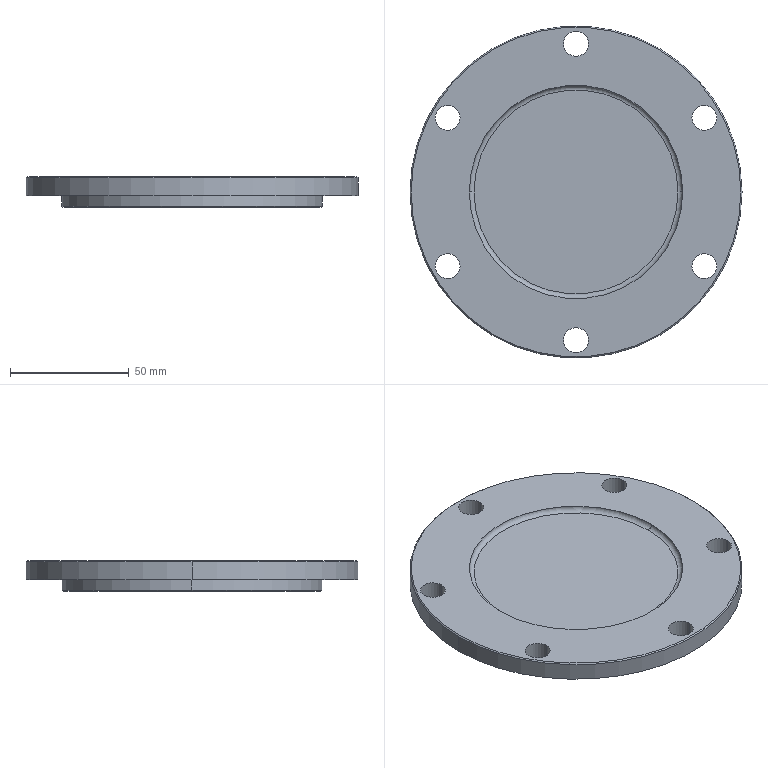Part | SolidWorks | features ICE 2, Chamfer 1, Extrusion 1, Fillet 1 | 1 solid | 29 faces | box 140 x 140 x 13 mm | volume 114660 mm3 | cylinder 18 | plane 5 | cone 4 | torus 2 | commonest cylinder face diameters 10.5 x12 100 x2 110 x2 140 x2
STEP:
#1=CARTESIAN_POINT('',(-43.,0.,6.));
#2=VERTEX_POINT('',#1);
#3=CARTESIAN_POINT('',(43.,0.,6.));
#4=VERTEX_POINT('',#3);
#5=CARTESIAN_POINT('',(0.,0.,6.));
#6=DIRECTION('',(0.,0.,1.));
#7=DIRECTION('',(1.,0.,0.));
#8=AXIS2_PLACEMENT_3D('',#5,#6,#7);
#9=CIRCLE('',#8,43.);
#10=EDGE_CURVE('',#2,#4,#9,.T.);
#11=ORIENTED_EDGE('',*,*,#10,.F.);
#12=CARTESIAN_POINT('',(-45.,0.,8.));
#13=VERTEX_POINT('',#12);
#14=CARTESIAN_POINT('',(-43.,0.,8.));
#15=DIRECTION('',(0.,1.,0.));
#16=DIRECTION('',(-1.,0.,0.));
#17=AXIS2_PLACEMENT_3D('',#14,#15,#16);
#18=CIRCLE('',#17,2.);
#19=EDGE_CURVE('',#2,#13,#18,.T.);
#20=ORIENTED_EDGE('',*,*,#19,.T.);
#21=CARTESIAN_POINT('',(45.,0.,8.));
#22=VERTEX_POINT('',#21);
#23=CARTESIAN_POINT('',(0.,0.,8.));
#24=DIRECTION('',(0.,0.,1.));
#25=DIRECTION('',(1.,0.,0.));
#26=AXIS2_PLACEMENT_3D('',#23,#24,#25);
#27=CIRCLE('',#26,45.);
#28=EDGE_CURVE('',#13,#22,#27,.T.);
#29=ORIENTED_EDGE('',*,*,#28,.T.);
#30=CARTESIAN_POINT('',(43.,0.,8.));
#31=DIRECTION('',(0.,-1.,0.));
#32=DIRECTION('',(0.,0.,-1.));
#33=AXIS2_PLACEMENT_3D('',#30,#31,#32);
#34=CIRCLE('',#33,2.);
#35=EDGE_CURVE('',#4,#22,#34,.T.);
#36=ORIENTED_EDGE('',*,*,#35,.F.);
#37=EDGE_LOOP('',(#11,#20,#29,#36));
#38=FACE_OUTER_BOUND('',#37,.T.);
#39=CARTESIAN_POINT('',(0.,0.,8.));
#40=DIRECTION('',(0.,0.,1.));
#41=DIRECTION('',(1.,0.,0.));
#42=AXIS2_PLACEMENT_3D('',#39,#40,#41);
#43=TOROIDAL_SURFACE('',#42,43.,2.);
#44=ADVANCED_FACE('',(#38),#43,.F.);
#45=CARTESIAN_POINT('',(69.5,0.,8.));
#46=VERTEX_POINT('',#45);
#47=CARTESIAN_POINT('',(-69.5,0.,8.));
#48=VERTEX_POINT('',#47);
#49=CARTESIAN_POINT('',(0.,0.,8.));
#50=DIRECTION('',(0.,0.,1.));
#51=DIRECTION('',(1.,0.,0.));
#52=AXIS2_PLACEMENT_3D('',#49,#50,#51);
#53=CIRCLE('',#52,69.5);
#54=EDGE_CURVE('',#46,#48,#53,.T.);
#55=ORIENTED_EDGE('',*,*,#54,.F.);
#56=CARTESIAN_POINT('',(70.,0.,7.5));
#57=VERTEX_POINT('',#56);
#58=CARTESIAN_POINT('',(69.5,0.,8.));
#59=DIRECTION('',(0.7071,0.,-0.7071));
#60=VECTOR('',#59,1000.);
#61=LINE('',#58,#60);
#62=EDGE_CURVE('',#46,#57,#61,.T.);
#63=ORIENTED_EDGE('',*,*,#62,.T.);
#64=CARTESIAN_POINT('',(-70.,0.,7.5));
#65=VERTEX_POINT('',#64);
#66=CARTESIAN_POINT('',(0.,0.,7.5));
#67=DIRECTION('',(0.,0.,-1.));
#68=DIRECTION('',(1.,0.,0.));
#69=AXIS2_PLACEMENT_3D('',#66,#67,#68);
#70=CIRCLE('',#69,70.);
#71=EDGE_CURVE('',#65,#57,#70,.T.);
#72=ORIENTED_EDGE('',*,*,#71,.F.);
#73=CARTESIAN_POINT('',(-69.5,0.,8.));
#74=DIRECTION('',(-0.7071,0.,-0.7071));
#75=VECTOR('',#74,1000.);
#76=LINE('',#73,#75);
#77=EDGE_CURVE('',#48,#65,#76,.T.);
#78=ORIENTED_EDGE('',*,*,#77,.F.);
#79=EDGE_LOOP('',(#55,#63,#72,#78));
#80=FACE_OUTER_BOUND('',#79,.T.);
#81=CARTESIAN_POINT('',(0.,0.,8.));
#82=DIRECTION('',(0.,0.,-1.));
#83=DIRECTION('',(-1.,0.,0.));
#84=AXIS2_PLACEMENT_3D('',#81,#82,#83);
#85=CONICAL_SURFACE('',#84,69.5,0.7854);
#86=ADVANCED_FACE('',(#80),#85,.T.);
#87=CARTESIAN_POINT('',(-54.5,0.,-5.));
#88=VERTEX_POINT('',#87);
#89=CARTESIAN_POINT('',(54.5,0.,-5.));
#90=VERTEX_POINT('',#89);
#91=CARTESIAN_POINT('',(0.,0.,-5.));
#92=DIRECTION('',(0.,0.,-1.));
#93=DIRECTION('',(-1.,0.,0.));
#94=AXIS2_PLACEMENT_3D('',#91,#92,#93);
#95=CIRCLE('',#94,54.5);
#96=EDGE_CURVE('',#88,#90,#95,.T.);
#97=ORIENTED_EDGE('',*,*,#96,.F.);
#98=CARTESIAN_POINT('',(-55.,0.,-4.5));
#99=VERTEX_POINT('',#98);
#100=CARTESIAN_POINT('',(-54.5,0.,-5.));
#101=DIRECTION('',(-0.7071,0.,0.7071));
#102=VECTOR('',#101,1000.);
#103=LINE('',#100,#102);
#104=EDGE_CURVE('',#88,#99,#103,.T.);
#105=ORIENTED_EDGE('',*,*,#104,.T.);
#106=CARTESIAN_POINT('',(55.,0.,-4.5));
#107=VERTEX_POINT('',#106);
#108=CARTESIAN_POINT('',(0.,0.,-4.5));
#109=DIRECTION('',(0.,0.,1.));
#110=DIRECTION('',(-1.,0.,0.));
#111=AXIS2_PLACEMENT_3D('',#108,#109,#110);
#112=CIRCLE('',#111,55.);
#113=EDGE_CURVE('',#107,#99,#112,.T.);
#114=ORIENTED_EDGE('',*,*,#113,.F.);
#115=CARTESIAN_POINT('',(54.5,0.,-5.));
#116=DIRECTION('',(0.7071,0.,0.7071));
#117=VECTOR('',#116,1000.);
#118=LINE('',#115,#117);
#119=EDGE_CURVE('',#90,#107,#118,.T.);
#120=ORIENTED_EDGE('',*,*,#119,.F.);
#121=EDGE_LOOP('',(#97,#105,#114,#120));
#122=FACE_OUTER_BOUND('',#121,.T.);
#123=CARTESIAN_POINT('',(0.,0.,-5.));
#124=DIRECTION('',(0.,0.,1.));
#125=DIRECTION('',(1.,0.,0.));
#126=AXIS2_PLACEMENT_3D('',#123,#124,#125);
#127=CONICAL_SURFACE('',#126,54.5,0.7854);
#128=ADVANCED_FACE('',(#122),#127,.T.);
#129=CARTESIAN_POINT('',(50.,0.,-5.));
#130=VERTEX_POINT('',#129);
#131=CARTESIAN_POINT('',(-50.,0.,-5.));
#132=VERTEX_POINT('',#131);
#133=CARTESIAN_POINT('',(0.,0.,-5.));
#134=DIRECTION('',(0.,0.,-1.));
#135=DIRECTION('',(-1.,0.,0.));
#136=AXIS2_PLACEMENT_3D('',#133,#134,#135);
#137=CIRCLE('',#136,50.);
#138=EDGE_CURVE('',#130,#132,#137,.T.);
#139=ORIENTED_EDGE('',*,*,#138,.T.);
#140=CARTESIAN_POINT('',(-50.,0.,0.));
#141=VERTEX_POINT('',#140);
#142=CARTESIAN_POINT('',(-50.,0.,-5.));
#143=DIRECTION('',(0.,0.,1.));
#144=VECTOR('',#143,1000.);
#145=LINE('',#142,#144);
#146=EDGE_CURVE('',#132,#141,#145,.T.);
#147=ORIENTED_EDGE('',*,*,#146,.T.);
#148=CARTESIAN_POINT('',(50.,0.,0.));
#149=VERTEX_POINT('',#148);
#150=CARTESIAN_POINT('',(0.,0.,0.));
#151=DIRECTION('',(0.,0.,-1.));
#152=DIRECTION('',(-1.,0.,0.));
#153=AXIS2_PLACEMENT_3D('',#150,#151,#152);
#154=CIRCLE('',#153,50.);
#155=EDGE_CURVE('',#149,#141,#154,.T.);
#156=ORIENTED_EDGE('',*,*,#155,.F.);
#157=CARTESIAN_POINT('',(50.,0.,-5.));
#158=DIRECTION('',(0.,0.,1.));
#159=VECTOR('',#158,1000.);
#160=LINE('',#157,#159);
#161=EDGE_CURVE('',#130,#149,#160,.T.);
#162=ORIENTED_EDGE('',*,*,#161,.F.);
#163=EDGE_LOOP('',(#139,#147,#156,#162));
#164=FACE_OUTER_BOUND('',#163,.T.);
#165=CARTESIAN_POINT('',(0.,0.,-5.));
#166=DIRECTION('',(0.,0.,1.));
#167=DIRECTION('',(1.,0.,0.));
#168=AXIS2_PLACEMENT_3D('',#165,#166,#167);
#169=CYLINDRICAL_SURFACE('',#168,50.);
#170=ADVANCED_FACE('',(#164),#169,.F.);
#171=ORIENTED_EDGE('',*,*,#113,.T.);
#172=CARTESIAN_POINT('',(-55.,0.,0.));
#173=VERTEX_POINT('',#172);
#174=CARTESIAN_POINT('',(-55.,0.,-5.));
#175=DIRECTION('',(0.,0.,1.));
#176=VECTOR('',#175,1000.);
#177=LINE('',#174,#176);
#178=EDGE_CURVE('',#99,#173,#177,.T.);
#179=ORIENTED_EDGE('',*,*,#178,.T.);
#180=CARTESIAN_POINT('',(55.,0.,0.));
#181=VERTEX_POINT('',#180);
#182=CARTESIAN_POINT('',(0.,0.,0.));
#183=DIRECTION('',(0.,0.,-1.));
#184=DIRECTION('',(1.,0.,0.));
#185=AXIS2_PLACEMENT_3D('',#182,#183,#184);
#186=CIRCLE('',#185,55.);
#187=EDGE_CURVE('',#173,#181,#186,.T.);
#188=ORIENTED_EDGE('',*,*,#187,.T.);
#189=CARTESIAN_POINT('',(55.,0.,-5.));
#190=DIRECTION('',(0.,0.,1.));
#191=VECTOR('',#190,1000.);
#192=LINE('',#189,#191);
#193=EDGE_CURVE('',#107,#181,#192,.T.);
#194=ORIENTED_EDGE('',*,*,#193,.F.);
#195=EDGE_LOOP('',(#171,#179,#188,#194));
#196=FACE_OUTER_BOUND('',#195,.T.);
#197=CARTESIAN_POINT('',(0.,0.,-5.));
#198=DIRECTION('',(0.,0.,1.));
#199=DIRECTION('',(1.,0.,0.));
#200=AXIS2_PLACEMENT_3D('',#197,#198,#199);
#201=CYLINDRICAL_SURFACE('',#200,55.);
#202=ADVANCED_FACE('',(#196),#201,.T.);
#203=CARTESIAN_POINT('',(-59.377,31.25,8.));
#204=VERTEX_POINT('',#203);
#205=CARTESIAN_POINT('',(-48.877,31.25,8.));
#206=VERTEX_POINT('',#205);
#207=CARTESIAN_POINT('',(-54.127,31.25,8.));
#208=DIRECTION('',(0.,0.,1.));
#209=DIRECTION('',(1.,0.,0.));
#210=AXIS2_PLACEMENT_3D('',#207,#208,#209);
#211=CIRCLE('',#210,5.25);
#212=EDGE_CURVE('',#204,#206,#211,.T.);
#213=ORIENTED_EDGE('',*,*,#212,.T.);
#214=CARTESIAN_POINT('',(-48.877,31.25,0.));
#215=VERTEX_POINT('',#214);
#216=CARTESIAN_POINT('',(-48.877,31.25,8.));
#217=DIRECTION('',(0.,0.,-1.));
#218=VECTOR('',#217,1000.);
#219=LINE('',#216,#218);
#220=EDGE_CURVE('',#206,#215,#219,.T.);
#221=ORIENTED_EDGE('',*,*,#220,.T.);
#222=CARTESIAN_POINT('',(-59.377,31.25,0.));
#223=VERTEX_POINT('',#222);
#224=CARTESIAN_POINT('',(-54.127,31.25,0.));
#225=DIRECTION('',(0.,0.,1.));
#226=DIRECTION('',(1.,0.,0.));
#227=AXIS2_PLACEMENT_3D('',#224,#225,#226);
#228=CIRCLE('',#227,5.25);
#229=EDGE_CURVE('',#223,#215,#228,.T.);
#230=ORIENTED_EDGE('',*,*,#229,.F.);
#231=CARTESIAN_POINT('',(-59.377,31.25,8.));
#232=DIRECTION('',(0.,0.,-1.));
#233=VECTOR('',#232,1000.);
#234=LINE('',#231,#233);
#235=EDGE_CURVE('',#204,#223,#234,.T.);
#236=ORIENTED_EDGE('',*,*,#235,.F.);
#237=EDGE_LOOP('',(#213,#221,#230,#236));
#238=FACE_OUTER_BOUND('',#237,.T.);
#239=CARTESIAN_POINT('',(-54.127,31.25,8.));
#240=DIRECTION('',(0.,0.,-1.));
#241=DIRECTION('',(-1.,0.,0.));
#242=AXIS2_PLACEMENT_3D('',#239,#240,#241);
#243=CYLINDRICAL_SURFACE('',#242,5.25);
#244=ADVANCED_FACE('',(#238),#243,.F.);
#245=CARTESIAN_POINT('',(-59.377,-31.25,8.));
#246=VERTEX_POINT('',#245);
#247=CARTESIAN_POINT('',(-48.877,-31.25,8.));
#248=VERTEX_POINT('',#247);
#249=CARTESIAN_POINT('',(-54.127,-31.25,8.));
#250=DIRECTION('',(0.,0.,1.));
#251=DIRECTION('',(1.,0.,0.));
#252=AXIS2_PLACEMENT_3D('',#249,#250,#251);
#253=CIRCLE('',#252,5.25);
#254=EDGE_CURVE('',#246,#248,#253,.T.);
#255=ORIENTED_EDGE('',*,*,#254,.T.);
#256=CARTESIAN_POINT('',(-48.877,-31.25,0.));
#257=VERTEX_POINT('',#256);
#258=CARTESIAN_POINT('',(-48.877,-31.25,8.));
#259=DIRECTION('',(0.,0.,-1.));
#260=VECTOR('',#259,1000.);
#261=LINE('',#258,#260);
#262=EDGE_CURVE('',#248,#257,#261,.T.);
#263=ORIENTED_EDGE('',*,*,#262,.T.);
#264=CARTESIAN_POINT('',(-59.377,-31.25,0.));
#265=VERTEX_POINT('',#264);
#266=CARTESIAN_POINT('',(-54.127,-31.25,0.));
#267=DIRECTION('',(0.,0.,1.));
#268=DIRECTION('',(1.,0.,0.));
#269=AXIS2_PLACEMENT_3D('',#266,#267,#268);
#270=CIRCLE('',#269,5.25);
#271=EDGE_CURVE('',#265,#257,#270,.T.);
#272=ORIENTED_EDGE('',*,*,#271,.F.);
#273=CARTESIAN_POINT('',(-59.377,-31.25,8.));
#274=DIRECTION('',(0.,0.,-1.));
#275=VECTOR('',#274,1000.);
#276=LINE('',#273,#275);
#277=EDGE_CURVE('',#246,#265,#276,.T.);
#278=ORIENTED_EDGE('',*,*,#277,.F.);
#279=EDGE_LOOP('',(#255,#263,#272,#278));
#280=FACE_OUTER_BOUND('',#279,.T.);
#281=CARTESIAN_POINT('',(-54.127,-31.25,8.));
#282=DIRECTION('',(0.,0.,-1.));
#283=DIRECTION('',(-1.,0.,0.));
#284=AXIS2_PLACEMENT_3D('',#281,#282,#283);
#285=CYLINDRICAL_SURFACE('',#284,5.25);
#286=ADVANCED_FACE('',(#280),#285,.F.);
#287=CARTESIAN_POINT('',(-5.25,-62.5,8.));
#288=VERTEX_POINT('',#287);
#289=CARTESIAN_POINT('',(5.25,-62.5,8.));
#290=VERTEX_POINT('',#289);
#291=CARTESIAN_POINT('',(0.,-62.5,8.));
#292=DIRECTION('',(0.,0.,1.));
#293=DIRECTION('',(1.,0.,0.));
#294=AXIS2_PLACEMENT_3D('',#291,#292,#293);
#295=CIRCLE('',#294,5.25);
#296=EDGE_CURVE('',#288,#290,#295,.T.);
#297=ORIENTED_EDGE('',*,*,#296,.T.);
#298=CARTESIAN_POINT('',(5.25,-62.5,0.));
#299=VERTEX_POINT('',#298);
#300=CARTESIAN_POINT('',(5.25,-62.5,8.));
#301=DIRECTION('',(0.,0.,-1.));
#302=VECTOR('',#301,1000.);
#303=LINE('',#300,#302);
#304=EDGE_CURVE('',#290,#299,#303,.T.);
#305=ORIENTED_EDGE('',*,*,#304,.T.);
#306=CARTESIAN_POINT('',(-5.25,-62.5,0.));
#307=VERTEX_POINT('',#306);
#308=CARTESIAN_POINT('',(0.,-62.5,0.));
#309=DIRECTION('',(0.,0.,1.));
#310=DIRECTION('',(1.,0.,0.));
#311=AXIS2_PLACEMENT_3D('',#308,#309,#310);
#312=CIRCLE('',#311,5.25);
#313=EDGE_CURVE('',#307,#299,#312,.T.);
#314=ORIENTED_EDGE('',*,*,#313,.F.);
#315=CARTESIAN_POINT('',(-5.25,-62.5,8.));
#316=DIRECTION('',(0.,0.,-1.));
#317=VECTOR('',#316,1000.);
#318=LINE('',#315,#317);
#319=EDGE_CURVE('',#288,#307,#318,.T.);
#320=ORIENTED_EDGE('',*,*,#319,.F.);
#321=EDGE_LOOP('',(#297,#305,#314,#320));
#322=FACE_OUTER_BOUND('',#321,.T.);
#323=CARTESIAN_POINT('',(0.,-62.5,8.));
#324=DIRECTION('',(0.,0.,-1.));
#325=DIRECTION('',(-1.,0.,0.));
#326=AXIS2_PLACEMENT_3D('',#323,#324,#325);
#327=CYLINDRICAL_SURFACE('',#326,5.25);
#328=ADVANCED_FACE('',(#322),#327,.F.);
#329=CARTESIAN_POINT('',(48.877,-31.25,8.));
#330=VERTEX_POINT('',#329);
#331=CARTESIAN_POINT('',(59.377,-31.25,8.));
#332=VERTEX_POINT('',#331);
#333=CARTESIAN_POINT('',(54.127,-31.25,8.));
#334=DIRECTION('',(0.,0.,1.));
#335=DIRECTION('',(1.,0.,0.));
#336=AXIS2_PLACEMENT_3D('',#333,#334,#335);
#337=CIRCLE('',#336,5.25);
#338=EDGE_CURVE('',#330,#332,#337,.T.);
#339=ORIENTED_EDGE('',*,*,#338,.T.);
#340=CARTESIAN_POINT('',(59.377,-31.25,0.));
#341=VERTEX_POINT('',#340);
#342=CARTESIAN_POINT('',(59.377,-31.25,8.));
#343=DIRECTION('',(0.,0.,-1.));
#344=VECTOR('',#343,1000.);
#345=LINE('',#342,#344);
#346=EDGE_CURVE('',#332,#341,#345,.T.);
#347=ORIENTED_EDGE('',*,*,#346,.T.);
#348=CARTESIAN_POINT('',(48.877,-31.25,0.));
#349=VERTEX_POINT('',#348);
#350=CARTESIAN_POINT('',(54.127,-31.25,0.));
#351=DIRECTION('',(0.,0.,1.));
#352=DIRECTION('',(1.,0.,0.));
#353=AXIS2_PLACEMENT_3D('',#350,#351,#352);
#354=CIRCLE('',#353,5.25);
#355=EDGE_CURVE('',#349,#341,#354,.T.);
#356=ORIENTED_EDGE('',*,*,#355,.F.);
#357=CARTESIAN_POINT('',(48.877,-31.25,8.));
#358=DIRECTION('',(0.,0.,-1.));
#359=VECTOR('',#358,1000.);
#360=LINE('',#357,#359);
#361=EDGE_CURVE('',#330,#349,#360,.T.);
#362=ORIENTED_EDGE('',*,*,#361,.F.);
#363=EDGE_LOOP('',(#339,#347,#356,#362));
#364=FACE_OUTER_BOUND('',#363,.T.);
#365=CARTESIAN_POINT('',(54.127,-31.25,8.));
#366=DIRECTION('',(0.,0.,-1.));
#367=DIRECTION('',(-1.,0.,0.));
#368=AXIS2_PLACEMENT_3D('',#365,#366,#367);
#369=CYLINDRICAL_SURFACE('',#368,5.25);
#370=ADVANCED_FACE('',(#364),#369,.F.);
#371=CARTESIAN_POINT('',(48.877,31.25,8.));
#372=VERTEX_POINT('',#371);
#373=CARTESIAN_POINT('',(59.377,31.25,8.));
#374=VERTEX_POINT('',#373);
#375=CARTESIAN_POINT('',(54.127,31.25,8.));
#376=DIRECTION('',(0.,0.,1.));
#377=DIRECTION('',(1.,0.,0.));
#378=AXIS2_PLACEMENT_3D('',#375,#376,#377);
#379=CIRCLE('',#378,5.25);
#380=EDGE_CURVE('',#372,#374,#379,.T.);
#381=ORIENTED_EDGE('',*,*,#380,.T.);
#382=CARTESIAN_POINT('',(59.377,31.25,0.));
#383=VERTEX_POINT('',#382);
#384=CARTESIAN_POINT('',(59.377,31.25,8.));
#385=DIRECTION('',(0.,0.,-1.));
#386=VECTOR('',#385,1000.);
#387=LINE('',#384,#386);
#388=EDGE_CURVE('',#374,#383,#387,.T.);
#389=ORIENTED_EDGE('',*,*,#388,.T.);
#390=CARTESIAN_POINT('',(48.877,31.25,0.));
#391=VERTEX_POINT('',#390);
#392=CARTESIAN_POINT('',(54.127,31.25,0.));
#393=DIRECTION('',(0.,0.,1.));
#394=DIRECTION('',(1.,0.,0.));
#395=AXIS2_PLACEMENT_3D('',#392,#393,#394);
#396=CIRCLE('',#395,5.25);
#397=EDGE_CURVE('',#391,#383,#396,.T.);
#398=ORIENTED_EDGE('',*,*,#397,.F.);
#399=CARTESIAN_POINT('',(48.877,31.25,8.));
#400=DIRECTION('',(0.,0.,-1.));
#401=VECTOR('',#400,1000.);
#402=LINE('',#399,#401);
#403=EDGE_CURVE('',#372,#391,#402,.T.);
#404=ORIENTED_EDGE('',*,*,#403,.F.);
#405=EDGE_LOOP('',(#381,#389,#398,#404));
#406=FACE_OUTER_BOUND('',#405,.T.);
#407=CARTESIAN_POINT('',(54.127,31.25,8.));
#408=DIRECTION('',(0.,0.,-1.));
#409=DIRECTION('',(-1.,0.,0.));
#410=AXIS2_PLACEMENT_3D('',#407,#408,#409);
#411=CYLINDRICAL_SURFACE('',#410,5.25);
#412=ADVANCED_FACE('',(#406),#411,.F.);
#413=CARTESIAN_POINT('',(-5.25,62.5,8.));
#414=VERTEX_POINT('',#413);
#415=CARTESIAN_POINT('',(5.25,62.5,8.));
#416=VERTEX_POINT('',#415);
#417=CARTESIAN_POINT('',(0.,62.5,8.));
#418=DIRECTION('',(0.,0.,1.));
#419=DIRECTION('',(1.,0.,0.));
#420=AXIS2_PLACEMENT_3D('',#417,#418,#419);
#421=CIRCLE('',#420,5.25);
#422=EDGE_CURVE('',#414,#416,#421,.T.);
#423=ORIENTED_EDGE('',*,*,#422,.T.);
#424=CARTESIAN_POINT('',(5.25,62.5,0.));
#425=VERTEX_POINT('',#424);
#426=CARTESIAN_POINT('',(5.25,62.5,8.));
#427=DIRECTION('',(0.,0.,-1.));
#428=VECTOR('',#427,1000.);
#429=LINE('',#426,#428);
#430=EDGE_CURVE('',#416,#425,#429,.T.);
#431=ORIENTED_EDGE('',*,*,#430,.T.);
#432=CARTESIAN_POINT('',(-5.25,62.5,0.));
#433=VERTEX_POINT('',#432);
#434=CARTESIAN_POINT('',(0.,62.5,0.));
#435=DIRECTION('',(0.,0.,1.));
#436=DIRECTION('',(1.,0.,0.));
#437=AXIS2_PLACEMENT_3D('',#434,#435,#436);
#438=CIRCLE('',#437,5.25);
#439=EDGE_CURVE('',#433,#425,#438,.T.);
#440=ORIENTED_EDGE('',*,*,#439,.F.);
#441=CARTESIAN_POINT('',(-5.25,62.5,8.));
#442=DIRECTION('',(0.,0.,-1.));
#443=VECTOR('',#442,1000.);
#444=LINE('',#441,#443);
#445=EDGE_CURVE('',#414,#433,#444,.T.);
#446=ORIENTED_EDGE('',*,*,#445,.F.);
#447=EDGE_LOOP('',(#423,#431,#440,#446));
#448=FACE_OUTER_BOUND('',#447,.T.);
#449=CARTESIAN_POINT('',(0.,62.5,8.));
#450=DIRECTION('',(0.,0.,-1.));
#451=DIRECTION('',(-1.,0.,0.));
#452=AXIS2_PLACEMENT_3D('',#449,#450,#451);
#453=CYLINDRICAL_SURFACE('',#452,5.25);
#454=ADVANCED_FACE('',(#448),#453,.F.);
#455=ORIENTED_EDGE('',*,*,#71,.T.);
#456=CARTESIAN_POINT('',(70.,0.,0.));
#457=VERTEX_POINT('',#456);
#458=CARTESIAN_POINT('',(70.,0.,8.));
#459=DIRECTION('',(0.,0.,-1.));
#460=VECTOR('',#459,1000.);
#461=LINE('',#458,#460);
#462=EDGE_CURVE('',#57,#457,#461,.T.);
#463=ORIENTED_EDGE('',*,*,#462,.T.);
#464=CARTESIAN_POINT('',(-70.,0.,0.));
#465=VERTEX_POINT('',#464);
#466=CARTESIAN_POINT('',(0.,0.,0.));
#467=DIRECTION('',(0.,0.,1.));
#468=DIRECTION('',(1.,0.,0.));
#469=AXIS2_PLACEMENT_3D('',#466,#467,#468);
#470=CIRCLE('',#469,70.);
#471=EDGE_CURVE('',#457,#465,#470,.T.);
#472=ORIENTED_EDGE('',*,*,#471,.T.);
#473=CARTESIAN_POINT('',(-70.,0.,8.));
#474=DIRECTION('',(0.,0.,-1.));
#475=VECTOR('',#474,1000.);
#476=LINE('',#473,#475);
#477=EDGE_CURVE('',#65,#465,#476,.T.);
#478=ORIENTED_EDGE('',*,*,#477,.F.);
#479=EDGE_LOOP('',(#455,#463,#472,#478));
#480=FACE_OUTER_BOUND('',#479,.T.);
#481=CARTESIAN_POINT('',(0.,0.,8.));
#482=DIRECTION('',(0.,0.,-1.));
#483=DIRECTION('',(-1.,0.,0.));
#484=AXIS2_PLACEMENT_3D('',#481,#482,#483);
#485=CYLINDRICAL_SURFACE('',#484,70.);
#486=ADVANCED_FACE('',(#480),#485,.T.);
#487=CARTESIAN_POINT('',(0.,0.,8.));
#488=DIRECTION('',(0.,0.,1.));
#489=DIRECTION('',(1.,0.,0.));
#490=AXIS2_PLACEMENT_3D('',#487,#488,#489);
#491=CIRCLE('',#490,45.);
#492=EDGE_CURVE('',#22,#13,#491,.T.);
#493=ORIENTED_EDGE('',*,*,#492,.F.);
#494=ORIENTED_EDGE('',*,*,#28,.F.);
#495=EDGE_LOOP('',(#493,#494));
#496=FACE_BOUND('',#495,.T.);
#497=CARTESIAN_POINT('',(0.,0.,8.));
#498=DIRECTION('',(0.,0.,1.));
#499=DIRECTION('',(1.,0.,0.));
#500=AXIS2_PLACEMENT_3D('',#497,#498,#499);
#501=CIRCLE('',#500,69.5);
#502=EDGE_CURVE('',#48,#46,#501,.T.);
#503=ORIENTED_EDGE('',*,*,#502,.T.);
#504=ORIENTED_EDGE('',*,*,#54,.T.);
#505=EDGE_LOOP('',(#503,#504));
#506=FACE_OUTER_BOUND('',#505,.T.);
#507=ORIENTED_EDGE('',*,*,#254,.F.);
#508=CARTESIAN_POINT('',(-54.127,-31.25,8.));
#509=DIRECTION('',(0.,0.,1.));
#510=DIRECTION('',(1.,0.,0.));
#511=AXIS2_PLACEMENT_3D('',#508,#509,#510);
#512=CIRCLE('',#511,5.25);
#513=EDGE_CURVE('',#248,#246,#512,.T.);
#514=ORIENTED_EDGE('',*,*,#513,.F.);
#515=EDGE_LOOP('',(#507,#514));
#516=FACE_BOUND('',#515,.T.);
#517=ORIENTED_EDGE('',*,*,#338,.F.);
#518=CARTESIAN_POINT('',(54.127,-31.25,8.));
#519=DIRECTION('',(0.,0.,1.));
#520=DIRECTION('',(1.,0.,0.));
#521=AXIS2_PLACEMENT_3D('',#518,#519,#520);
#522=CIRCLE('',#521,5.25);
#523=EDGE_CURVE('',#332,#330,#522,.T.);
#524=ORIENTED_EDGE('',*,*,#523,.F.);
#525=EDGE_LOOP('',(#517,#524));
#526=FACE_BOUND('',#525,.T.);
#527=ORIENTED_EDGE('',*,*,#422,.F.);
#528=CARTESIAN_POINT('',(0.,62.5,8.));
#529=DIRECTION('',(0.,0.,1.));
#530=DIRECTION('',(1.,0.,0.));
#531=AXIS2_PLACEMENT_3D('',#528,#529,#530);
#532=CIRCLE('',#531,5.25);
#533=EDGE_CURVE('',#416,#414,#532,.T.);
#534=ORIENTED_EDGE('',*,*,#533,.F.);
#535=EDGE_LOOP('',(#527,#534));
#536=FACE_BOUND('',#535,.T.);
#537=ORIENTED_EDGE('',*,*,#380,.F.);
#538=CARTESIAN_POINT('',(54.127,31.25,8.));
#539=DIRECTION('',(0.,0.,1.));
#540=DIRECTION('',(1.,0.,0.));
#541=AXIS2_PLACEMENT_3D('',#538,#539,#540);
#542=CIRCLE('',#541,5.25);
#543=EDGE_CURVE('',#374,#372,#542,.T.);
#544=ORIENTED_EDGE('',*,*,#543,.F.);
#545=EDGE_LOOP('',(#537,#544));
#546=FACE_BOUND('',#545,.T.);
#547=ORIENTED_EDGE('',*,*,#296,.F.);
#548=CARTESIAN_POINT('',(0.,-62.5,8.));
#549=DIRECTION('',(0.,0.,1.));
#550=DIRECTION('',(1.,0.,0.));
#551=AXIS2_PLACEMENT_3D('',#548,#549,#550);
#552=CIRCLE('',#551,5.25);
#553=EDGE_CURVE('',#290,#288,#552,.T.);
#554=ORIENTED_EDGE('',*,*,#553,.F.);
#555=EDGE_LOOP('',(#547,#554));
#556=FACE_BOUND('',#555,.T.);
#557=ORIENTED_EDGE('',*,*,#212,.F.);
#558=CARTESIAN_POINT('',(-54.127,31.25,8.));
#559=DIRECTION('',(0.,0.,1.));
#560=DIRECTION('',(1.,0.,0.));
#561=AXIS2_PLACEMENT_3D('',#558,#559,#560);
#562=CIRCLE('',#561,5.25);
#563=EDGE_CURVE('',#206,#204,#562,.T.);
#564=ORIENTED_EDGE('',*,*,#563,.F.);
#565=EDGE_LOOP('',(#557,#564));
#566=FACE_BOUND('',#565,.T.);
#567=CARTESIAN_POINT('',(0.,0.,8.));
#568=DIRECTION('',(0.,0.,1.));
#569=DIRECTION('',(1.,0.,0.));
#570=AXIS2_PLACEMENT_3D('',#567,#568,#569);
#571=PLANE('',#570);
#572=ADVANCED_FACE('',(#496,#506,#516,#526,#536,#546,#556,#566),#571,.T.);
#573=CARTESIAN_POINT('',(0.,0.,0.));
#574=DIRECTION('',(0.,0.,-1.));
#575=DIRECTION('',(1.,0.,0.));
#576=AXIS2_PLACEMENT_3D('',#573,#574,#575);
#577=CIRCLE('',#576,55.);
#578=EDGE_CURVE('',#181,#173,#577,.T.);
#579=ORIENTED_EDGE('',*,*,#578,.F.);
#580=ORIENTED_EDGE('',*,*,#187,.F.);
#581=EDGE_LOOP('',(#579,#580));
#582=FACE_BOUND('',#581,.T.);
#583=CARTESIAN_POINT('',(0.,0.,0.));
#584=DIRECTION('',(0.,0.,1.));
#585=DIRECTION('',(1.,0.,0.));
#586=AXIS2_PLACEMENT_3D('',#583,#584,#585);
#587=CIRCLE('',#586,70.);
#588=EDGE_CURVE('',#465,#457,#587,.T.);
#589=ORIENTED_EDGE('',*,*,#588,.F.);
#590=ORIENTED_EDGE('',*,*,#471,.F.);
#591=EDGE_LOOP('',(#589,#590));
#592=FACE_OUTER_BOUND('',#591,.T.);
#593=ORIENTED_EDGE('',*,*,#439,.T.);
#594=CARTESIAN_POINT('',(0.,62.5,0.));
#595=DIRECTION('',(0.,0.,1.));
#596=DIRECTION('',(1.,0.,0.));
#597=AXIS2_PLACEMENT_3D('',#594,#595,#596);
#598=CIRCLE('',#597,5.25);
#599=EDGE_CURVE('',#425,#433,#598,.T.);
#600=ORIENTED_EDGE('',*,*,#599,.T.);
#601=EDGE_LOOP('',(#593,#600));
#602=FACE_BOUND('',#601,.T.);
#603=ORIENTED_EDGE('',*,*,#397,.T.);
#604=CARTESIAN_POINT('',(54.127,31.25,0.));
#605=DIRECTION('',(0.,0.,1.));
#606=DIRECTION('',(1.,0.,0.));
#607=AXIS2_PLACEMENT_3D('',#604,#605,#606);
#608=CIRCLE('',#607,5.25);
#609=EDGE_CURVE('',#383,#391,#608,.T.);
#610=ORIENTED_EDGE('',*,*,#609,.T.);
#611=EDGE_LOOP('',(#603,#610));
#612=FACE_BOUND('',#611,.T.);
#613=ORIENTED_EDGE('',*,*,#355,.T.);
#614=CARTESIAN_POINT('',(54.127,-31.25,0.));
#615=DIRECTION('',(0.,0.,1.));
#616=DIRECTION('',(1.,0.,0.));
#617=AXIS2_PLACEMENT_3D('',#614,#615,#616);
#618=CIRCLE('',#617,5.25);
#619=EDGE_CURVE('',#341,#349,#618,.T.);
#620=ORIENTED_EDGE('',*,*,#619,.T.);
#621=EDGE_LOOP('',(#613,#620));
#622=FACE_BOUND('',#621,.T.);
#623=ORIENTED_EDGE('',*,*,#313,.T.);
#624=CARTESIAN_POINT('',(0.,-62.5,0.));
#625=DIRECTION('',(0.,0.,1.));
#626=DIRECTION('',(1.,0.,0.));
#627=AXIS2_PLACEMENT_3D('',#624,#625,#626);
#628=CIRCLE('',#627,5.25);
#629=EDGE_CURVE('',#299,#307,#628,.T.);
#630=ORIENTED_EDGE('',*,*,#629,.T.);
#631=EDGE_LOOP('',(#623,#630));
#632=FACE_BOUND('',#631,.T.);
#633=ORIENTED_EDGE('',*,*,#271,.T.);
#634=CARTESIAN_POINT('',(-54.127,-31.25,0.));
#635=DIRECTION('',(0.,0.,1.));
#636=DIRECTION('',(1.,0.,0.));
#637=AXIS2_PLACEMENT_3D('',#634,#635,#636);
#638=CIRCLE('',#637,5.25);
#639=EDGE_CURVE('',#257,#265,#638,.T.);
#640=ORIENTED_EDGE('',*,*,#639,.T.);
#641=EDGE_LOOP('',(#633,#640));
#642=FACE_BOUND('',#641,.T.);
#643=ORIENTED_EDGE('',*,*,#229,.T.);
#644=CARTESIAN_POINT('',(-54.127,31.25,0.));
#645=DIRECTION('',(0.,0.,1.));
#646=DIRECTION('',(1.,0.,0.));
#647=AXIS2_PLACEMENT_3D('',#644,#645,#646);
#648=CIRCLE('',#647,5.25);
#649=EDGE_CURVE('',#215,#223,#648,.T.);
#650=ORIENTED_EDGE('',*,*,#649,.T.);
#651=EDGE_LOOP('',(#643,#650));
#652=FACE_BOUND('',#651,.T.);
#653=CARTESIAN_POINT('',(0.,0.,0.));
#654=DIRECTION('',(0.,0.,1.));
#655=DIRECTION('',(1.,0.,0.));
#656=AXIS2_PLACEMENT_3D('',#653,#654,#655);
#657=PLANE('',#656);
#658=ADVANCED_FACE('',(#582,#592,#602,#612,#622,#632,#642,#652),#657,.F.);
#659=ORIENTED_EDGE('',*,*,#462,.F.);
#660=CARTESIAN_POINT('',(0.,0.,7.5));
#661=DIRECTION('',(0.,0.,-1.));
#662=DIRECTION('',(1.,0.,0.));
#663=AXIS2_PLACEMENT_3D('',#660,#661,#662);
#664=CIRCLE('',#663,70.);
#665=EDGE_CURVE('',#57,#65,#664,.T.);
#666=ORIENTED_EDGE('',*,*,#665,.T.);
#667=ORIENTED_EDGE('',*,*,#477,.T.);
#668=ORIENTED_EDGE('',*,*,#588,.T.);
#669=EDGE_LOOP('',(#659,#666,#667,#668));
#670=FACE_OUTER_BOUND('',#669,.T.);
#671=CARTESIAN_POINT('',(0.,0.,8.));
#672=DIRECTION('',(0.,0.,-1.));
#673=DIRECTION('',(-1.,0.,0.));
#674=AXIS2_PLACEMENT_3D('',#671,#672,#673);
#675=CYLINDRICAL_SURFACE('',#674,70.);
#676=ADVANCED_FACE('',(#670),#675,.T.);
#677=ORIENTED_EDGE('',*,*,#430,.F.);
#678=ORIENTED_EDGE('',*,*,#533,.T.);
#679=ORIENTED_EDGE('',*,*,#445,.T.);
#680=ORIENTED_EDGE('',*,*,#599,.F.);
#681=EDGE_LOOP('',(#677,#678,#679,#680));
#682=FACE_OUTER_BOUND('',#681,.T.);
#683=CARTESIAN_POINT('',(0.,62.5,8.));
#684=DIRECTION('',(0.,0.,-1.));
#685=DIRECTION('',(-1.,0.,0.));
#686=AXIS2_PLACEMENT_3D('',#683,#684,#685);
#687=CYLINDRICAL_SURFACE('',#686,5.25);
#688=ADVANCED_FACE('',(#682),#687,.F.);
#689=ORIENTED_EDGE('',*,*,#388,.F.);
#690=ORIENTED_EDGE('',*,*,#543,.T.);
#691=ORIENTED_EDGE('',*,*,#403,.T.);
#692=ORIENTED_EDGE('',*,*,#609,.F.);
#693=EDGE_LOOP('',(#689,#690,#691,#692));
#694=FACE_OUTER_BOUND('',#693,.T.);
#695=CARTESIAN_POINT('',(54.127,31.25,8.));
#696=DIRECTION('',(0.,0.,-1.));
#697=DIRECTION('',(-1.,0.,0.));
#698=AXIS2_PLACEMENT_3D('',#695,#696,#697);
#699=CYLINDRICAL_SURFACE('',#698,5.25);
#700=ADVANCED_FACE('',(#694),#699,.F.);
#701=ORIENTED_EDGE('',*,*,#346,.F.);
#702=ORIENTED_EDGE('',*,*,#523,.T.);
#703=ORIENTED_EDGE('',*,*,#361,.T.);
#704=ORIENTED_EDGE('',*,*,#619,.F.);
#705=EDGE_LOOP('',(#701,#702,#703,#704));
#706=FACE_OUTER_BOUND('',#705,.T.);
#707=CARTESIAN_POINT('',(54.127,-31.25,8.));
#708=DIRECTION('',(0.,0.,-1.));
#709=DIRECTION('',(-1.,0.,0.));
#710=AXIS2_PLACEMENT_3D('',#707,#708,#709);
#711=CYLINDRICAL_SURFACE('',#710,5.25);
#712=ADVANCED_FACE('',(#706),#711,.F.);
#713=ORIENTED_EDGE('',*,*,#304,.F.);
#714=ORIENTED_EDGE('',*,*,#553,.T.);
#715=ORIENTED_EDGE('',*,*,#319,.T.);
#716=ORIENTED_EDGE('',*,*,#629,.F.);
#717=EDGE_LOOP('',(#713,#714,#715,#716));
#718=FACE_OUTER_BOUND('',#717,.T.);
#719=CARTESIAN_POINT('',(0.,-62.5,8.));
#720=DIRECTION('',(0.,0.,-1.));
#721=DIRECTION('',(-1.,0.,0.));
#722=AXIS2_PLACEMENT_3D('',#719,#720,#721);
#723=CYLINDRICAL_SURFACE('',#722,5.25);
#724=ADVANCED_FACE('',(#718),#723,.F.);
#725=ORIENTED_EDGE('',*,*,#262,.F.);
#726=ORIENTED_EDGE('',*,*,#513,.T.);
#727=ORIENTED_EDGE('',*,*,#277,.T.);
#728=ORIENTED_EDGE('',*,*,#639,.F.);
#729=EDGE_LOOP('',(#725,#726,#727,#728));
#730=FACE_OUTER_BOUND('',#729,.T.);
#731=CARTESIAN_POINT('',(-54.127,-31.25,8.));
#732=DIRECTION('',(0.,0.,-1.));
#733=DIRECTION('',(-1.,0.,0.));
#734=AXIS2_PLACEMENT_3D('',#731,#732,#733);
#735=CYLINDRICAL_SURFACE('',#734,5.25);
#736=ADVANCED_FACE('',(#730),#735,.F.);
#737=ORIENTED_EDGE('',*,*,#220,.F.);
#738=ORIENTED_EDGE('',*,*,#563,.T.);
#739=ORIENTED_EDGE('',*,*,#235,.T.);
#740=ORIENTED_EDGE('',*,*,#649,.F.);
#741=EDGE_LOOP('',(#737,#738,#739,#740));
#742=FACE_OUTER_BOUND('',#741,.T.);
#743=CARTESIAN_POINT('',(-54.127,31.25,8.));
#744=DIRECTION('',(0.,0.,-1.));
#745=DIRECTION('',(-1.,0.,0.));
#746=AXIS2_PLACEMENT_3D('',#743,#744,#745);
#747=CYLINDRICAL_SURFACE('',#746,5.25);
#748=ADVANCED_FACE('',(#742),#747,.F.);
#749=CARTESIAN_POINT('',(0.,0.,-5.));
#750=DIRECTION('',(0.,0.,-1.));
#751=DIRECTION('',(-1.,0.,0.));
#752=AXIS2_PLACEMENT_3D('',#749,#750,#751);
#753=CIRCLE('',#752,54.5);
#754=EDGE_CURVE('',#90,#88,#753,.T.);
#755=ORIENTED_EDGE('',*,*,#754,.T.);
#756=ORIENTED_EDGE('',*,*,#96,.T.);
#757=EDGE_LOOP('',(#755,#756));
#758=FACE_OUTER_BOUND('',#757,.T.);
#759=ORIENTED_EDGE('',*,*,#138,.F.);
#760=CARTESIAN_POINT('',(0.,0.,-5.));
#761=DIRECTION('',(0.,0.,-1.));
#762=DIRECTION('',(-1.,0.,0.));
#763=AXIS2_PLACEMENT_3D('',#760,#761,#762);
#764=CIRCLE('',#763,50.);
#765=EDGE_CURVE('',#132,#130,#764,.T.);
#766=ORIENTED_EDGE('',*,*,#765,.F.);
#767=EDGE_LOOP('',(#759,#766));
#768=FACE_BOUND('',#767,.T.);
#769=CARTESIAN_POINT('',(0.,0.,-5.));
#770=DIRECTION('',(0.,0.,-1.));
#771=DIRECTION('',(-1.,0.,0.));
#772=AXIS2_PLACEMENT_3D('',#769,#770,#771);
#773=PLANE('',#772);
#774=ADVANCED_FACE('',(#758,#768),#773,.T.);
#775=ORIENTED_EDGE('',*,*,#178,.F.);
#776=CARTESIAN_POINT('',(0.,0.,-4.5));
#777=DIRECTION('',(0.,0.,1.));
#778=DIRECTION('',(-1.,0.,0.));
#779=AXIS2_PLACEMENT_3D('',#776,#777,#778);
#780=CIRCLE('',#779,55.);
#781=EDGE_CURVE('',#99,#107,#780,.T.);
#782=ORIENTED_EDGE('',*,*,#781,.T.);
#783=ORIENTED_EDGE('',*,*,#193,.T.);
#784=ORIENTED_EDGE('',*,*,#578,.T.);
#785=EDGE_LOOP('',(#775,#782,#783,#784));
#786=FACE_OUTER_BOUND('',#785,.T.);
#787=CARTESIAN_POINT('',(0.,0.,-5.));
#788=DIRECTION('',(0.,0.,1.));
#789=DIRECTION('',(1.,0.,0.));
#790=AXIS2_PLACEMENT_3D('',#787,#788,#789);
#791=CYLINDRICAL_SURFACE('',#790,55.);
#792=ADVANCED_FACE('',(#786),#791,.T.);
#793=ORIENTED_EDGE('',*,*,#146,.F.);
#794=ORIENTED_EDGE('',*,*,#765,.T.);
#795=ORIENTED_EDGE('',*,*,#161,.T.);
#796=CARTESIAN_POINT('',(0.,0.,0.));
#797=DIRECTION('',(0.,0.,-1.));
#798=DIRECTION('',(-1.,0.,0.));
#799=AXIS2_PLACEMENT_3D('',#796,#797,#798);
#800=CIRCLE('',#799,50.);
#801=EDGE_CURVE('',#141,#149,#800,.T.);
#802=ORIENTED_EDGE('',*,*,#801,.F.);
#803=EDGE_LOOP('',(#793,#794,#795,#802));
#804=FACE_OUTER_BOUND('',#803,.T.);
#805=CARTESIAN_POINT('',(0.,0.,-5.));
#806=DIRECTION('',(0.,0.,1.));
#807=DIRECTION('',(1.,0.,0.));
#808=AXIS2_PLACEMENT_3D('',#805,#806,#807);
#809=CYLINDRICAL_SURFACE('',#808,50.);
#810=ADVANCED_FACE('',(#804),#809,.F.);
#811=ORIENTED_EDGE('',*,*,#155,.T.);
#812=ORIENTED_EDGE('',*,*,#801,.T.);
#813=EDGE_LOOP('',(#811,#812));
#814=FACE_OUTER_BOUND('',#813,.T.);
#815=CARTESIAN_POINT('',(0.,0.,0.));
#816=DIRECTION('',(0.,0.,1.));
#817=DIRECTION('',(1.,0.,0.));
#818=AXIS2_PLACEMENT_3D('',#815,#816,#817);
#819=PLANE('',#818);
#820=ADVANCED_FACE('',(#814),#819,.F.);
#821=ORIENTED_EDGE('',*,*,#104,.F.);
#822=ORIENTED_EDGE('',*,*,#754,.F.);
#823=ORIENTED_EDGE('',*,*,#119,.T.);
#824=ORIENTED_EDGE('',*,*,#781,.F.);
#825=EDGE_LOOP('',(#821,#822,#823,#824));
#826=FACE_OUTER_BOUND('',#825,.T.);
#827=CARTESIAN_POINT('',(0.,0.,-5.));
#828=DIRECTION('',(0.,0.,1.));
#829=DIRECTION('',(1.,0.,0.));
#830=AXIS2_PLACEMENT_3D('',#827,#828,#829);
#831=CONICAL_SURFACE('',#830,54.5,0.7854);
#832=ADVANCED_FACE('',(#826),#831,.T.);
#833=ORIENTED_EDGE('',*,*,#62,.F.);
#834=ORIENTED_EDGE('',*,*,#502,.F.);
#835=ORIENTED_EDGE('',*,*,#77,.T.);
#836=ORIENTED_EDGE('',*,*,#665,.F.);
#837=EDGE_LOOP('',(#833,#834,#835,#836));
#838=FACE_OUTER_BOUND('',#837,.T.);
#839=CARTESIAN_POINT('',(0.,0.,8.));
#840=DIRECTION('',(0.,0.,-1.));
#841=DIRECTION('',(-1.,0.,0.));
#842=AXIS2_PLACEMENT_3D('',#839,#840,#841);
#843=CONICAL_SURFACE('',#842,69.5,0.7854);
#844=ADVANCED_FACE('',(#838),#843,.T.);
#845=CARTESIAN_POINT('',(0.,0.,6.));
#846=DIRECTION('',(0.,0.,1.));
#847=DIRECTION('',(1.,0.,0.));
#848=AXIS2_PLACEMENT_3D('',#845,#846,#847);
#849=CIRCLE('',#848,43.);
#850=EDGE_CURVE('',#4,#2,#849,.T.);
#851=ORIENTED_EDGE('',*,*,#850,.T.);
#852=ORIENTED_EDGE('',*,*,#10,.T.);
#853=EDGE_LOOP('',(#851,#852));
#854=FACE_OUTER_BOUND('',#853,.T.);
#855=CARTESIAN_POINT('',(0.,0.,6.));
#856=DIRECTION('',(0.,0.,1.));
#857=DIRECTION('',(1.,0.,0.));
#858=AXIS2_PLACEMENT_3D('',#855,#856,#857);
#859=PLANE('',#858);
#860=ADVANCED_FACE('',(#854),#859,.T.);
#861=ORIENTED_EDGE('',*,*,#19,.F.);
#862=ORIENTED_EDGE('',*,*,#850,.F.);
#863=ORIENTED_EDGE('',*,*,#35,.T.);
#864=ORIENTED_EDGE('',*,*,#492,.T.);
#865=EDGE_LOOP('',(#861,#862,#863,#864));
#866=FACE_OUTER_BOUND('',#865,.T.);
#867=CARTESIAN_POINT('',(0.,0.,8.));
#868=DIRECTION('',(0.,0.,1.));
#869=DIRECTION('',(1.,0.,0.));
#870=AXIS2_PLACEMENT_3D('',#867,#868,#869);
#871=TOROIDAL_SURFACE('',#870,43.,2.);
#872=ADVANCED_FACE('',(#866),#871,.F.);
#873=CLOSED_SHELL('',(#44,#86,#128,#170,#202,#244,#286,#328,#370,#412,#454,#486,#572,#658,#676,#688,#700,#712,#724,#736,#748,#774,#792,#810,#820,#832,#844,#860,#872));
#874=MANIFOLD_SOLID_BREP('',#873);
#875=CARTESIAN_POINT('',(0.,0.,0.));
#876=DIRECTION('',(0.,0.,1.));
#877=DIRECTION('',(1.,0.,0.));
#878=AXIS2_PLACEMENT_3D('',#875,#876,#877);
#879=(LENGTH_UNIT()NAMED_UNIT(*)SI_UNIT(.MILLI.,.METRE.));
#880=UNCERTAINTY_MEASURE_WITH_UNIT(LENGTH_MEASURE(0.00001),#879,'','');
#881=(NAMED_UNIT(*)PLANE_ANGLE_UNIT()SI_UNIT($,.RADIAN.));
#882=(NAMED_UNIT(*)SI_UNIT($,.STERADIAN.)SOLID_ANGLE_UNIT());
#883=(GEOMETRIC_REPRESENTATION_CONTEXT(3)GLOBAL_UNCERTAINTY_ASSIGNED_CONTEXT((#880))GLOBAL_UNIT_ASSIGNED_CONTEXT((#879,#881,#882))REPRESENTATION_CONTEXT('',''));
#884=ADVANCED_BREP_SHAPE_REPRESENTATION('',(#874,#878),#883);